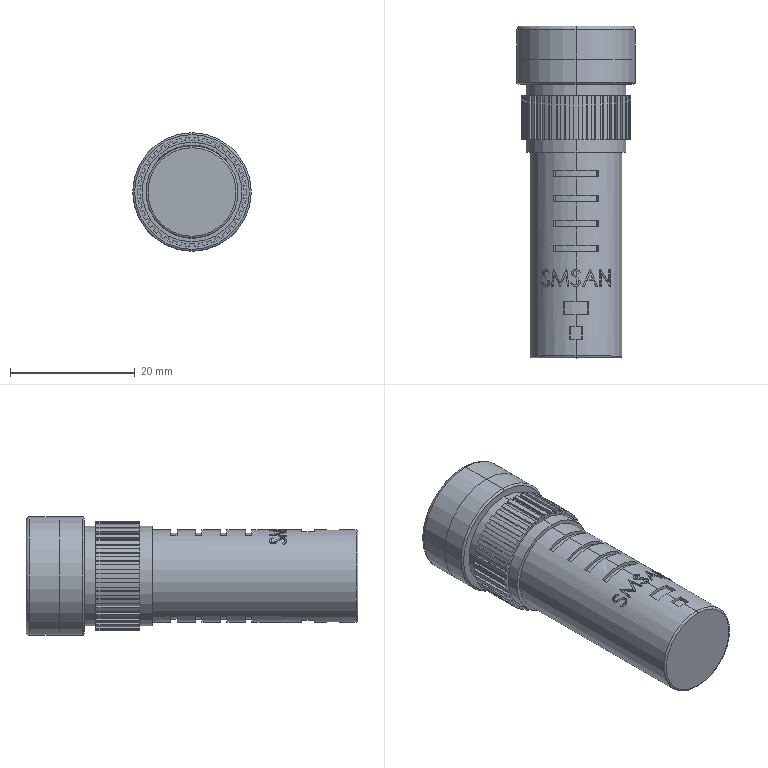Part | SolidWorks | features BaseBody 2 | 2 solids | 319 faces | box 19 x 53.2 x 19 mm | volume 10652 mm3 | plane 150 | cylinder 113 | spline 50 | torus 6 | commonest cylinder face diameters 16.6 x39 17.5 x38 13.8 x18 14.8 x5 15 x5 16 x4